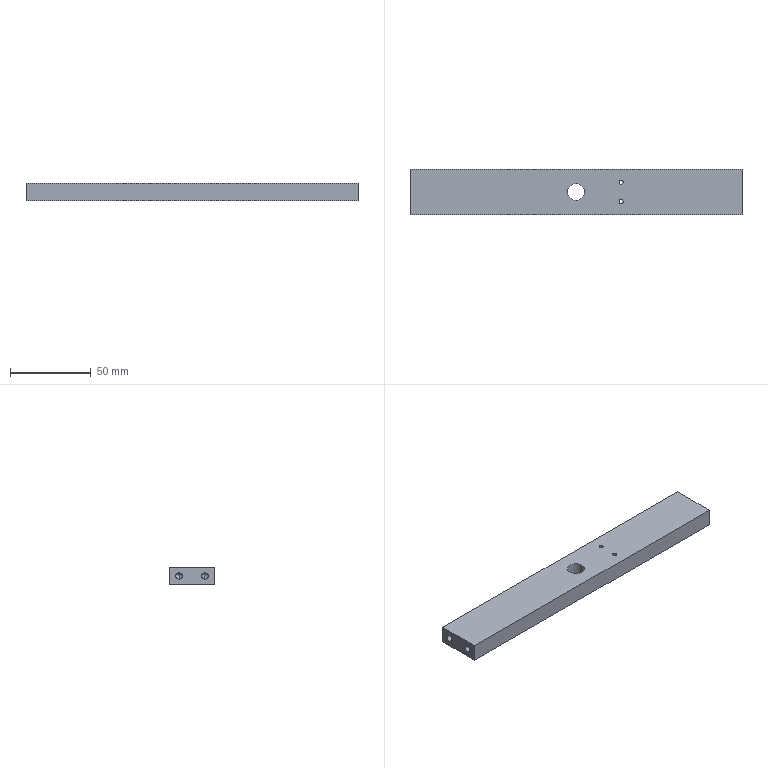Part | STEP file | PN_0020 (pull block) | 1 solid | 28 faces | box 206 x 28 x 11 mm | volume 61677 mm3 | cylinder 14 | cone 8 | plane 6 | commonest cylinder face diameters 4.2 x8 2.5 x4 10.5 x2